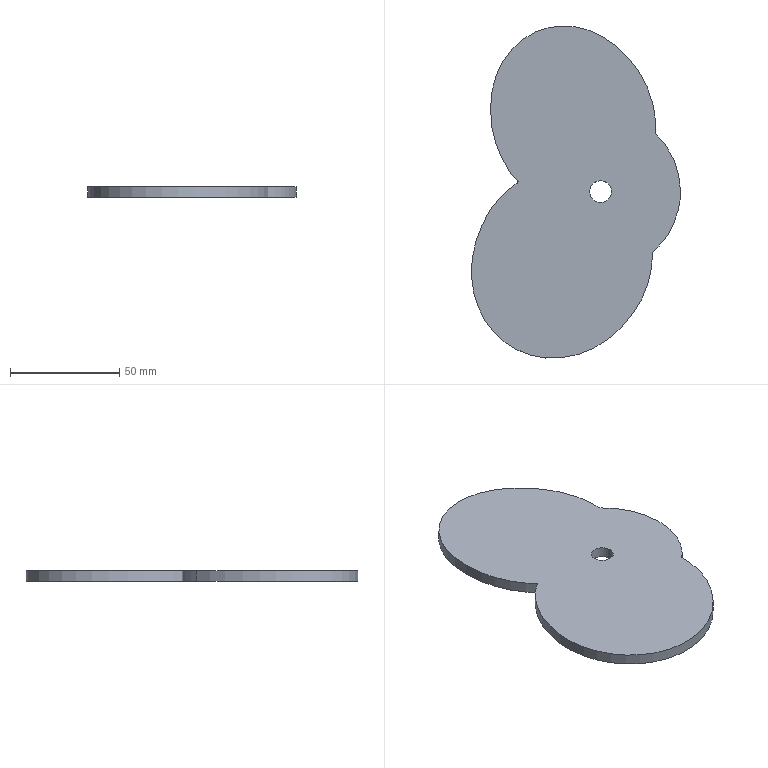Part | SolidWorks | features CurveInFile 1, Extrusion 1, ICE 1 | 1 solid | 6 faces | box 95.852 x 152.391 x 5 mm | volume 53303 mm3 | cylinder 2 | spline 2 | plane 2 | commonest cylinder face diameters 10 x2